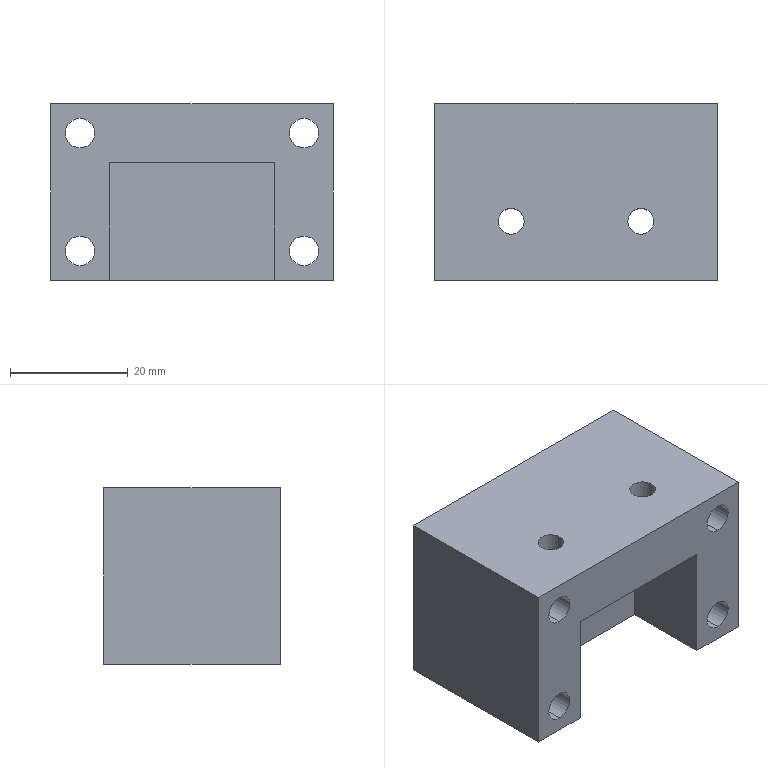Part | SolidWorks | features ICE 3, Extrusion 1 | 1 solid | 22 faces | box 48 x 30 x 30 mm | volume 32140 mm3 | cylinder 12 | plane 10 | commonest cylinder face diameters 5 x8 4.4 x4
STEP:
#1=CARTESIAN_POINT('',(0.01845,0.01653,0.0025));
#2=VERTEX_POINT('',#1);
#3=CARTESIAN_POINT('',(0.01845,0.01653,0.0075));
#4=VERTEX_POINT('',#3);
#5=CARTESIAN_POINT('',(0.01845,0.01653,0.005));
#6=DIRECTION('',(0.,1.,0.));
#7=DIRECTION('',(0.,0.,-1.));
#8=AXIS2_PLACEMENT_3D('',#5,#6,#7);
#9=CIRCLE('',#8,0.0025);
#10=EDGE_CURVE('',#2,#4,#9,.T.);
#11=ORIENTED_EDGE('',*,*,#10,.T.);
#12=CARTESIAN_POINT('',(0.01845,-0.01347,0.0075));
#13=VERTEX_POINT('',#12);
#14=CARTESIAN_POINT('',(0.01845,0.0236,0.0075));
#15=DIRECTION('',(0.,-1.,0.));
#16=VECTOR('',#15,1.);
#17=LINE('',#14,#16);
#18=EDGE_CURVE('',#4,#13,#17,.T.);
#19=ORIENTED_EDGE('',*,*,#18,.T.);
#20=CARTESIAN_POINT('',(0.01845,-0.01347,0.0025));
#21=VERTEX_POINT('',#20);
#22=CARTESIAN_POINT('',(0.01845,-0.01347,0.005));
#23=DIRECTION('',(0.,-1.,0.));
#24=DIRECTION('',(0.,0.,-1.));
#25=AXIS2_PLACEMENT_3D('',#22,#23,#24);
#26=CIRCLE('',#25,0.0025);
#27=EDGE_CURVE('',#13,#21,#26,.T.);
#28=ORIENTED_EDGE('',*,*,#27,.T.);
#29=CARTESIAN_POINT('',(0.01845,0.0236,0.0025));
#30=DIRECTION('',(0.,-1.,0.));
#31=VECTOR('',#30,1.);
#32=LINE('',#29,#31);
#33=EDGE_CURVE('',#2,#21,#32,.T.);
#34=ORIENTED_EDGE('',*,*,#33,.F.);
#35=EDGE_LOOP('',(#11,#19,#28,#34));
#36=FACE_OUTER_BOUND('',#35,.T.);
#37=CARTESIAN_POINT('',(0.01845,0.0236,0.005));
#38=DIRECTION('',(0.,-1.,0.));
#39=DIRECTION('',(0.,0.,-1.));
#40=AXIS2_PLACEMENT_3D('',#37,#38,#39);
#41=CYLINDRICAL_SURFACE('',#40,0.0025);
#42=ADVANCED_FACE('',(#36),#41,.F.);
#43=CARTESIAN_POINT('',(0.01845,0.01653,0.0225));
#44=VERTEX_POINT('',#43);
#45=CARTESIAN_POINT('',(0.01845,0.01653,0.0275));
#46=VERTEX_POINT('',#45);
#47=CARTESIAN_POINT('',(0.01845,0.01653,0.025));
#48=DIRECTION('',(0.,1.,0.));
#49=DIRECTION('',(0.,0.,-1.));
#50=AXIS2_PLACEMENT_3D('',#47,#48,#49);
#51=CIRCLE('',#50,0.0025);
#52=EDGE_CURVE('',#44,#46,#51,.T.);
#53=ORIENTED_EDGE('',*,*,#52,.T.);
#54=CARTESIAN_POINT('',(0.01845,-0.01347,0.0275));
#55=VERTEX_POINT('',#54);
#56=CARTESIAN_POINT('',(0.01845,0.0236,0.0275));
#57=DIRECTION('',(0.,-1.,0.));
#58=VECTOR('',#57,1.);
#59=LINE('',#56,#58);
#60=EDGE_CURVE('',#46,#55,#59,.T.);
#61=ORIENTED_EDGE('',*,*,#60,.T.);
#62=CARTESIAN_POINT('',(0.01845,-0.01347,0.0225));
#63=VERTEX_POINT('',#62);
#64=CARTESIAN_POINT('',(0.01845,-0.01347,0.025));
#65=DIRECTION('',(0.,-1.,0.));
#66=DIRECTION('',(0.,0.,-1.));
#67=AXIS2_PLACEMENT_3D('',#64,#65,#66);
#68=CIRCLE('',#67,0.0025);
#69=EDGE_CURVE('',#55,#63,#68,.T.);
#70=ORIENTED_EDGE('',*,*,#69,.T.);
#71=CARTESIAN_POINT('',(0.01845,0.0236,0.0225));
#72=DIRECTION('',(0.,-1.,0.));
#73=VECTOR('',#72,1.);
#74=LINE('',#71,#73);
#75=EDGE_CURVE('',#44,#63,#74,.T.);
#76=ORIENTED_EDGE('',*,*,#75,.F.);
#77=EDGE_LOOP('',(#53,#61,#70,#76));
#78=FACE_OUTER_BOUND('',#77,.T.);
#79=CARTESIAN_POINT('',(0.01845,0.0236,0.025));
#80=DIRECTION('',(0.,-1.,0.));
#81=DIRECTION('',(0.,0.,-1.));
#82=AXIS2_PLACEMENT_3D('',#79,#80,#81);
#83=CYLINDRICAL_SURFACE('',#82,0.0025);
#84=ADVANCED_FACE('',(#78),#83,.F.);
#85=CARTESIAN_POINT('',(-0.01955,0.01653,0.0225));
#86=VERTEX_POINT('',#85);
#87=CARTESIAN_POINT('',(-0.01955,0.01653,0.0275));
#88=VERTEX_POINT('',#87);
#89=CARTESIAN_POINT('',(-0.01955,0.01653,0.025));
#90=DIRECTION('',(0.,1.,0.));
#91=DIRECTION('',(0.,0.,-1.));
#92=AXIS2_PLACEMENT_3D('',#89,#90,#91);
#93=CIRCLE('',#92,0.0025);
#94=EDGE_CURVE('',#86,#88,#93,.T.);
#95=ORIENTED_EDGE('',*,*,#94,.T.);
#96=CARTESIAN_POINT('',(-0.01955,-0.01347,0.0275));
#97=VERTEX_POINT('',#96);
#98=CARTESIAN_POINT('',(-0.01955,0.0236,0.0275));
#99=DIRECTION('',(0.,-1.,0.));
#100=VECTOR('',#99,1.);
#101=LINE('',#98,#100);
#102=EDGE_CURVE('',#88,#97,#101,.T.);
#103=ORIENTED_EDGE('',*,*,#102,.T.);
#104=CARTESIAN_POINT('',(-0.01955,-0.01347,0.0225));
#105=VERTEX_POINT('',#104);
#106=CARTESIAN_POINT('',(-0.01955,-0.01347,0.025));
#107=DIRECTION('',(0.,-1.,0.));
#108=DIRECTION('',(0.,0.,-1.));
#109=AXIS2_PLACEMENT_3D('',#106,#107,#108);
#110=CIRCLE('',#109,0.0025);
#111=EDGE_CURVE('',#97,#105,#110,.T.);
#112=ORIENTED_EDGE('',*,*,#111,.T.);
#113=CARTESIAN_POINT('',(-0.01955,0.0236,0.0225));
#114=DIRECTION('',(0.,-1.,0.));
#115=VECTOR('',#114,1.);
#116=LINE('',#113,#115);
#117=EDGE_CURVE('',#86,#105,#116,.T.);
#118=ORIENTED_EDGE('',*,*,#117,.F.);
#119=EDGE_LOOP('',(#95,#103,#112,#118));
#120=FACE_OUTER_BOUND('',#119,.T.);
#121=CARTESIAN_POINT('',(-0.01955,0.0236,0.025));
#122=DIRECTION('',(0.,-1.,0.));
#123=DIRECTION('',(0.,0.,-1.));
#124=AXIS2_PLACEMENT_3D('',#121,#122,#123);
#125=CYLINDRICAL_SURFACE('',#124,0.0025);
#126=ADVANCED_FACE('',(#120),#125,.F.);
#127=CARTESIAN_POINT('',(-0.01955,0.01653,0.0025));
#128=VERTEX_POINT('',#127);
#129=CARTESIAN_POINT('',(-0.01955,0.01653,0.0075));
#130=VERTEX_POINT('',#129);
#131=CARTESIAN_POINT('',(-0.01955,0.01653,0.005));
#132=DIRECTION('',(0.,1.,0.));
#133=DIRECTION('',(0.,0.,-1.));
#134=AXIS2_PLACEMENT_3D('',#131,#132,#133);
#135=CIRCLE('',#134,0.0025);
#136=EDGE_CURVE('',#128,#130,#135,.T.);
#137=ORIENTED_EDGE('',*,*,#136,.T.);
#138=CARTESIAN_POINT('',(-0.01955,-0.01347,0.0075));
#139=VERTEX_POINT('',#138);
#140=CARTESIAN_POINT('',(-0.01955,0.0236,0.0075));
#141=DIRECTION('',(0.,-1.,0.));
#142=VECTOR('',#141,1.);
#143=LINE('',#140,#142);
#144=EDGE_CURVE('',#130,#139,#143,.T.);
#145=ORIENTED_EDGE('',*,*,#144,.T.);
#146=CARTESIAN_POINT('',(-0.01955,-0.01347,0.0025));
#147=VERTEX_POINT('',#146);
#148=CARTESIAN_POINT('',(-0.01955,-0.01347,0.005));
#149=DIRECTION('',(0.,-1.,0.));
#150=DIRECTION('',(0.,0.,-1.));
#151=AXIS2_PLACEMENT_3D('',#148,#149,#150);
#152=CIRCLE('',#151,0.0025);
#153=EDGE_CURVE('',#139,#147,#152,.T.);
#154=ORIENTED_EDGE('',*,*,#153,.T.);
#155=CARTESIAN_POINT('',(-0.01955,0.0236,0.0025));
#156=DIRECTION('',(0.,-1.,0.));
#157=VECTOR('',#156,1.);
#158=LINE('',#155,#157);
#159=EDGE_CURVE('',#128,#147,#158,.T.);
#160=ORIENTED_EDGE('',*,*,#159,.F.);
#161=EDGE_LOOP('',(#137,#145,#154,#160));
#162=FACE_OUTER_BOUND('',#161,.T.);
#163=CARTESIAN_POINT('',(-0.01955,0.0236,0.005));
#164=DIRECTION('',(0.,-1.,0.));
#165=DIRECTION('',(0.,0.,-1.));
#166=AXIS2_PLACEMENT_3D('',#163,#164,#165);
#167=CYLINDRICAL_SURFACE('',#166,0.0025);
#168=ADVANCED_FACE('',(#162),#167,.F.);
#169=CARTESIAN_POINT('',(0.008255,-0.003473,0.03));
#170=VERTEX_POINT('',#169);
#171=CARTESIAN_POINT('',(0.01265,-0.003473,0.03));
#172=VERTEX_POINT('',#171);
#173=CARTESIAN_POINT('',(0.01045,-0.003473,0.03));
#174=DIRECTION('',(0.,0.,1.));
#175=DIRECTION('',(1.,0.,0.));
#176=AXIS2_PLACEMENT_3D('',#173,#174,#175);
#177=CIRCLE('',#176,0.0022);
#178=EDGE_CURVE('',#170,#172,#177,.T.);
#179=ORIENTED_EDGE('',*,*,#178,.T.);
#180=CARTESIAN_POINT('',(0.01265,-0.003473,0.02));
#181=VERTEX_POINT('',#180);
#182=CARTESIAN_POINT('',(0.01265,-0.003473,0.04));
#183=DIRECTION('',(0.,0.,-1.));
#184=VECTOR('',#183,1.);
#185=LINE('',#182,#184);
#186=EDGE_CURVE('',#172,#181,#185,.T.);
#187=ORIENTED_EDGE('',*,*,#186,.T.);
#188=CARTESIAN_POINT('',(0.008255,-0.003473,0.02));
#189=VERTEX_POINT('',#188);
#190=CARTESIAN_POINT('',(0.01045,-0.003473,0.02));
#191=DIRECTION('',(0.,0.,-1.));
#192=DIRECTION('',(-1.,0.,0.));
#193=AXIS2_PLACEMENT_3D('',#190,#191,#192);
#194=CIRCLE('',#193,0.0022);
#195=EDGE_CURVE('',#181,#189,#194,.T.);
#196=ORIENTED_EDGE('',*,*,#195,.T.);
#197=CARTESIAN_POINT('',(0.008255,-0.003473,0.04));
#198=DIRECTION('',(0.,0.,-1.));
#199=VECTOR('',#198,1.);
#200=LINE('',#197,#199);
#201=EDGE_CURVE('',#170,#189,#200,.T.);
#202=ORIENTED_EDGE('',*,*,#201,.F.);
#203=EDGE_LOOP('',(#179,#187,#196,#202));
#204=FACE_OUTER_BOUND('',#203,.T.);
#205=CARTESIAN_POINT('',(0.01045,-0.003473,0.04));
#206=DIRECTION('',(0.,0.,-1.));
#207=DIRECTION('',(-1.,0.,0.));
#208=AXIS2_PLACEMENT_3D('',#205,#206,#207);
#209=CYLINDRICAL_SURFACE('',#208,0.0022);
#210=ADVANCED_FACE('',(#204),#209,.F.);
#211=CARTESIAN_POINT('',(-0.01375,-0.003473,0.03));
#212=VERTEX_POINT('',#211);
#213=CARTESIAN_POINT('',(-0.009345,-0.003473,0.03));
#214=VERTEX_POINT('',#213);
#215=CARTESIAN_POINT('',(-0.01155,-0.003473,0.03));
#216=DIRECTION('',(0.,0.,1.));
#217=DIRECTION('',(1.,0.,0.));
#218=AXIS2_PLACEMENT_3D('',#215,#216,#217);
#219=CIRCLE('',#218,0.0022);
#220=EDGE_CURVE('',#212,#214,#219,.T.);
#221=ORIENTED_EDGE('',*,*,#220,.T.);
#222=CARTESIAN_POINT('',(-0.009345,-0.003473,0.02));
#223=VERTEX_POINT('',#222);
#224=CARTESIAN_POINT('',(-0.009345,-0.003473,0.04));
#225=DIRECTION('',(0.,0.,-1.));
#226=VECTOR('',#225,1.);
#227=LINE('',#224,#226);
#228=EDGE_CURVE('',#214,#223,#227,.T.);
#229=ORIENTED_EDGE('',*,*,#228,.T.);
#230=CARTESIAN_POINT('',(-0.01375,-0.003473,0.02));
#231=VERTEX_POINT('',#230);
#232=CARTESIAN_POINT('',(-0.01155,-0.003473,0.02));
#233=DIRECTION('',(0.,0.,-1.));
#234=DIRECTION('',(-1.,0.,0.));
#235=AXIS2_PLACEMENT_3D('',#232,#233,#234);
#236=CIRCLE('',#235,0.0022);
#237=EDGE_CURVE('',#223,#231,#236,.T.);
#238=ORIENTED_EDGE('',*,*,#237,.T.);
#239=CARTESIAN_POINT('',(-0.01375,-0.003473,0.04));
#240=DIRECTION('',(0.,0.,-1.));
#241=VECTOR('',#240,1.);
#242=LINE('',#239,#241);
#243=EDGE_CURVE('',#212,#231,#242,.T.);
#244=ORIENTED_EDGE('',*,*,#243,.F.);
#245=EDGE_LOOP('',(#221,#229,#238,#244));
#246=FACE_OUTER_BOUND('',#245,.T.);
#247=CARTESIAN_POINT('',(-0.01155,-0.003473,0.04));
#248=DIRECTION('',(0.,0.,-1.));
#249=DIRECTION('',(-1.,0.,0.));
#250=AXIS2_PLACEMENT_3D('',#247,#248,#249);
#251=CYLINDRICAL_SURFACE('',#250,0.0022);
#252=ADVANCED_FACE('',(#246),#251,.F.);
#253=CARTESIAN_POINT('',(-0.02455,0.01653,0.));
#254=VERTEX_POINT('',#253);
#255=CARTESIAN_POINT('',(-0.02455,-0.01347,0.));
#256=VERTEX_POINT('',#255);
#257=CARTESIAN_POINT('',(-0.02455,0.01653,0.));
#258=DIRECTION('',(0.,-1.,0.));
#259=VECTOR('',#258,1.);
#260=LINE('',#257,#259);
#261=EDGE_CURVE('',#254,#256,#260,.T.);
#262=ORIENTED_EDGE('',*,*,#261,.T.);
#263=CARTESIAN_POINT('',(-0.02455,-0.01347,0.03));
#264=VERTEX_POINT('',#263);
#265=CARTESIAN_POINT('',(-0.02455,-0.01347,0.03));
#266=DIRECTION('',(0.,0.,-1.));
#267=VECTOR('',#266,1.);
#268=LINE('',#265,#267);
#269=EDGE_CURVE('',#264,#256,#268,.T.);
#270=ORIENTED_EDGE('',*,*,#269,.F.);
#271=CARTESIAN_POINT('',(-0.02455,0.01653,0.03));
#272=VERTEX_POINT('',#271);
#273=CARTESIAN_POINT('',(-0.02455,0.01653,0.03));
#274=DIRECTION('',(0.,-1.,0.));
#275=VECTOR('',#274,1.);
#276=LINE('',#273,#275);
#277=EDGE_CURVE('',#272,#264,#276,.T.);
#278=ORIENTED_EDGE('',*,*,#277,.F.);
#279=CARTESIAN_POINT('',(-0.02455,0.01653,0.03));
#280=DIRECTION('',(0.,0.,-1.));
#281=VECTOR('',#280,1.);
#282=LINE('',#279,#281);
#283=EDGE_CURVE('',#272,#254,#282,.T.);
#284=ORIENTED_EDGE('',*,*,#283,.T.);
#285=EDGE_LOOP('',(#262,#270,#278,#284));
#286=FACE_OUTER_BOUND('',#285,.T.);
#287=CARTESIAN_POINT('',(-0.02455,0.01653,0.03));
#288=DIRECTION('',(1.,0.,0.));
#289=DIRECTION('',(0.,1.,0.));
#290=AXIS2_PLACEMENT_3D('',#287,#288,#289);
#291=PLANE('',#290);
#292=ADVANCED_FACE('',(#286),#291,.F.);
#293=CARTESIAN_POINT('',(0.01845,-0.01347,0.005));
#294=DIRECTION('',(0.,-1.,0.));
#295=DIRECTION('',(0.,0.,-1.));
#296=AXIS2_PLACEMENT_3D('',#293,#294,#295);
#297=CIRCLE('',#296,0.0025);
#298=EDGE_CURVE('',#21,#13,#297,.T.);
#299=ORIENTED_EDGE('',*,*,#298,.F.);
#300=ORIENTED_EDGE('',*,*,#27,.F.);
#301=EDGE_LOOP('',(#299,#300));
#302=FACE_BOUND('',#301,.T.);
#303=CARTESIAN_POINT('',(0.01845,-0.01347,0.025));
#304=DIRECTION('',(0.,-1.,0.));
#305=DIRECTION('',(0.,0.,-1.));
#306=AXIS2_PLACEMENT_3D('',#303,#304,#305);
#307=CIRCLE('',#306,0.0025);
#308=EDGE_CURVE('',#63,#55,#307,.T.);
#309=ORIENTED_EDGE('',*,*,#308,.F.);
#310=ORIENTED_EDGE('',*,*,#69,.F.);
#311=EDGE_LOOP('',(#309,#310));
#312=FACE_BOUND('',#311,.T.);
#313=CARTESIAN_POINT('',(-0.01955,-0.01347,0.025));
#314=DIRECTION('',(0.,-1.,0.));
#315=DIRECTION('',(0.,0.,-1.));
#316=AXIS2_PLACEMENT_3D('',#313,#314,#315);
#317=CIRCLE('',#316,0.0025);
#318=EDGE_CURVE('',#105,#97,#317,.T.);
#319=ORIENTED_EDGE('',*,*,#318,.F.);
#320=ORIENTED_EDGE('',*,*,#111,.F.);
#321=EDGE_LOOP('',(#319,#320));
#322=FACE_BOUND('',#321,.T.);
#323=CARTESIAN_POINT('',(-0.01955,-0.01347,0.005));
#324=DIRECTION('',(0.,-1.,0.));
#325=DIRECTION('',(0.,0.,-1.));
#326=AXIS2_PLACEMENT_3D('',#323,#324,#325);
#327=CIRCLE('',#326,0.0025);
#328=EDGE_CURVE('',#147,#139,#327,.T.);
#329=ORIENTED_EDGE('',*,*,#328,.F.);
#330=ORIENTED_EDGE('',*,*,#153,.F.);
#331=EDGE_LOOP('',(#329,#330));
#332=FACE_BOUND('',#331,.T.);
#333=CARTESIAN_POINT('',(0.01345,-0.01347,0.02));
#334=VERTEX_POINT('',#333);
#335=CARTESIAN_POINT('',(-0.01455,-0.01347,0.02));
#336=VERTEX_POINT('',#335);
#337=CARTESIAN_POINT('',(0.01345,-0.01347,0.02));
#338=DIRECTION('',(-1.,0.,0.));
#339=VECTOR('',#338,1.);
#340=LINE('',#337,#339);
#341=EDGE_CURVE('',#334,#336,#340,.T.);
#342=ORIENTED_EDGE('',*,*,#341,.F.);
#343=CARTESIAN_POINT('',(0.01345,-0.01347,0.));
#344=VERTEX_POINT('',#343);
#345=CARTESIAN_POINT('',(0.01345,-0.01347,0.02));
#346=DIRECTION('',(0.,0.,-1.));
#347=VECTOR('',#346,1.);
#348=LINE('',#345,#347);
#349=EDGE_CURVE('',#334,#344,#348,.T.);
#350=ORIENTED_EDGE('',*,*,#349,.T.);
#351=CARTESIAN_POINT('',(0.02345,-0.01347,0.));
#352=VERTEX_POINT('',#351);
#353=CARTESIAN_POINT('',(-0.02455,-0.01347,0.));
#354=DIRECTION('',(1.,0.,0.));
#355=VECTOR('',#354,1.);
#356=LINE('',#353,#355);
#357=EDGE_CURVE('',#344,#352,#356,.T.);
#358=ORIENTED_EDGE('',*,*,#357,.T.);
#359=CARTESIAN_POINT('',(0.02345,-0.01347,0.03));
#360=VERTEX_POINT('',#359);
#361=CARTESIAN_POINT('',(0.02345,-0.01347,0.03));
#362=DIRECTION('',(0.,0.,-1.));
#363=VECTOR('',#362,1.);
#364=LINE('',#361,#363);
#365=EDGE_CURVE('',#360,#352,#364,.T.);
#366=ORIENTED_EDGE('',*,*,#365,.F.);
#367=CARTESIAN_POINT('',(-0.02455,-0.01347,0.03));
#368=DIRECTION('',(1.,0.,0.));
#369=VECTOR('',#368,1.);
#370=LINE('',#367,#369);
#371=EDGE_CURVE('',#264,#360,#370,.T.);
#372=ORIENTED_EDGE('',*,*,#371,.F.);
#373=ORIENTED_EDGE('',*,*,#269,.T.);
#374=CARTESIAN_POINT('',(-0.01455,-0.01347,0.));
#375=VERTEX_POINT('',#374);
#376=CARTESIAN_POINT('',(-0.02455,-0.01347,0.));
#377=DIRECTION('',(1.,0.,0.));
#378=VECTOR('',#377,1.);
#379=LINE('',#376,#378);
#380=EDGE_CURVE('',#256,#375,#379,.T.);
#381=ORIENTED_EDGE('',*,*,#380,.T.);
#382=CARTESIAN_POINT('',(-0.01455,-0.01347,0.02));
#383=DIRECTION('',(0.,0.,-1.));
#384=VECTOR('',#383,1.);
#385=LINE('',#382,#384);
#386=EDGE_CURVE('',#336,#375,#385,.T.);
#387=ORIENTED_EDGE('',*,*,#386,.F.);
#388=EDGE_LOOP('',(#342,#350,#358,#366,#372,#373,#381,#387));
#389=FACE_OUTER_BOUND('',#388,.T.);
#390=CARTESIAN_POINT('',(-0.02455,-0.01347,0.03));
#391=DIRECTION('',(0.,1.,0.));
#392=DIRECTION('',(0.,0.,1.));
#393=AXIS2_PLACEMENT_3D('',#390,#391,#392);
#394=PLANE('',#393);
#395=ADVANCED_FACE('',(#302,#312,#322,#332,#389),#394,.F.);
#396=CARTESIAN_POINT('',(0.02345,0.01653,0.));
#397=VERTEX_POINT('',#396);
#398=CARTESIAN_POINT('',(0.02345,0.01653,0.));
#399=DIRECTION('',(0.,1.,0.));
#400=VECTOR('',#399,1.);
#401=LINE('',#398,#400);
#402=EDGE_CURVE('',#352,#397,#401,.T.);
#403=ORIENTED_EDGE('',*,*,#402,.T.);
#404=CARTESIAN_POINT('',(0.02345,0.01653,0.03));
#405=VERTEX_POINT('',#404);
#406=CARTESIAN_POINT('',(0.02345,0.01653,0.03));
#407=DIRECTION('',(0.,0.,-1.));
#408=VECTOR('',#407,1.);
#409=LINE('',#406,#408);
#410=EDGE_CURVE('',#405,#397,#409,.T.);
#411=ORIENTED_EDGE('',*,*,#410,.F.);
#412=CARTESIAN_POINT('',(0.02345,0.01653,0.03));
#413=DIRECTION('',(0.,1.,0.));
#414=VECTOR('',#413,1.);
#415=LINE('',#412,#414);
#416=EDGE_CURVE('',#360,#405,#415,.T.);
#417=ORIENTED_EDGE('',*,*,#416,.F.);
#418=ORIENTED_EDGE('',*,*,#365,.T.);
#419=EDGE_LOOP('',(#403,#411,#417,#418));
#420=FACE_OUTER_BOUND('',#419,.T.);
#421=CARTESIAN_POINT('',(0.02345,0.01653,0.03));
#422=DIRECTION('',(-1.,0.,0.));
#423=DIRECTION('',(0.,-1.,0.));
#424=AXIS2_PLACEMENT_3D('',#421,#422,#423);
#425=PLANE('',#424);
#426=ADVANCED_FACE('',(#420),#425,.F.);
#427=ORIENTED_EDGE('',*,*,#10,.F.);
#428=CARTESIAN_POINT('',(0.01845,0.01653,0.005));
#429=DIRECTION('',(0.,1.,0.));
#430=DIRECTION('',(0.,0.,-1.));
#431=AXIS2_PLACEMENT_3D('',#428,#429,#430);
#432=CIRCLE('',#431,0.0025);
#433=EDGE_CURVE('',#4,#2,#432,.T.);
#434=ORIENTED_EDGE('',*,*,#433,.F.);
#435=EDGE_LOOP('',(#427,#434));
#436=FACE_BOUND('',#435,.T.);
#437=ORIENTED_EDGE('',*,*,#52,.F.);
#438=CARTESIAN_POINT('',(0.01845,0.01653,0.025));
#439=DIRECTION('',(0.,1.,0.));
#440=DIRECTION('',(0.,0.,-1.));
#441=AXIS2_PLACEMENT_3D('',#438,#439,#440);
#442=CIRCLE('',#441,0.0025);
#443=EDGE_CURVE('',#46,#44,#442,.T.);
#444=ORIENTED_EDGE('',*,*,#443,.F.);
#445=EDGE_LOOP('',(#437,#444));
#446=FACE_BOUND('',#445,.T.);
#447=ORIENTED_EDGE('',*,*,#94,.F.);
#448=CARTESIAN_POINT('',(-0.01955,0.01653,0.025));
#449=DIRECTION('',(0.,1.,0.));
#450=DIRECTION('',(0.,0.,-1.));
#451=AXIS2_PLACEMENT_3D('',#448,#449,#450);
#452=CIRCLE('',#451,0.0025);
#453=EDGE_CURVE('',#88,#86,#452,.T.);
#454=ORIENTED_EDGE('',*,*,#453,.F.);
#455=EDGE_LOOP('',(#447,#454));
#456=FACE_BOUND('',#455,.T.);
#457=ORIENTED_EDGE('',*,*,#136,.F.);
#458=CARTESIAN_POINT('',(-0.01955,0.01653,0.005));
#459=DIRECTION('',(0.,1.,0.));
#460=DIRECTION('',(0.,0.,-1.));
#461=AXIS2_PLACEMENT_3D('',#458,#459,#460);
#462=CIRCLE('',#461,0.0025);
#463=EDGE_CURVE('',#130,#128,#462,.T.);
#464=ORIENTED_EDGE('',*,*,#463,.F.);
#465=EDGE_LOOP('',(#457,#464));
#466=FACE_BOUND('',#465,.T.);
#467=CARTESIAN_POINT('',(-0.02455,0.01653,0.));
#468=DIRECTION('',(-1.,0.,0.));
#469=VECTOR('',#468,1.);
#470=LINE('',#467,#469);
#471=EDGE_CURVE('',#397,#254,#470,.T.);
#472=ORIENTED_EDGE('',*,*,#471,.T.);
#473=ORIENTED_EDGE('',*,*,#283,.F.);
#474=CARTESIAN_POINT('',(-0.02455,0.01653,0.03));
#475=DIRECTION('',(-1.,0.,0.));
#476=VECTOR('',#475,1.);
#477=LINE('',#474,#476);
#478=EDGE_CURVE('',#405,#272,#477,.T.);
#479=ORIENTED_EDGE('',*,*,#478,.F.);
#480=ORIENTED_EDGE('',*,*,#410,.T.);
#481=EDGE_LOOP('',(#472,#473,#479,#480));
#482=FACE_OUTER_BOUND('',#481,.T.);
#483=CARTESIAN_POINT('',(-0.02455,0.01653,0.03));
#484=DIRECTION('',(0.,-1.,0.));
#485=DIRECTION('',(0.,0.,-1.));
#486=AXIS2_PLACEMENT_3D('',#483,#484,#485);
#487=PLANE('',#486);
#488=ADVANCED_FACE('',(#436,#446,#456,#466,#482),#487,.F.);
#489=ORIENTED_EDGE('',*,*,#178,.F.);
#490=CARTESIAN_POINT('',(0.01045,-0.003473,0.03));
#491=DIRECTION('',(0.,0.,1.));
#492=DIRECTION('',(1.,0.,0.));
#493=AXIS2_PLACEMENT_3D('',#490,#491,#492);
#494=CIRCLE('',#493,0.0022);
#495=EDGE_CURVE('',#172,#170,#494,.T.);
#496=ORIENTED_EDGE('',*,*,#495,.F.);
#497=EDGE_LOOP('',(#489,#496));
#498=FACE_BOUND('',#497,.T.);
#499=ORIENTED_EDGE('',*,*,#220,.F.);
#500=CARTESIAN_POINT('',(-0.01155,-0.003473,0.03));
#501=DIRECTION('',(0.,0.,1.));
#502=DIRECTION('',(1.,0.,0.));
#503=AXIS2_PLACEMENT_3D('',#500,#501,#502);
#504=CIRCLE('',#503,0.0022);
#505=EDGE_CURVE('',#214,#212,#504,.T.);
#506=ORIENTED_EDGE('',*,*,#505,.F.);
#507=EDGE_LOOP('',(#499,#506));
#508=FACE_BOUND('',#507,.T.);
#509=ORIENTED_EDGE('',*,*,#277,.T.);
#510=ORIENTED_EDGE('',*,*,#371,.T.);
#511=ORIENTED_EDGE('',*,*,#416,.T.);
#512=ORIENTED_EDGE('',*,*,#478,.T.);
#513=EDGE_LOOP('',(#509,#510,#511,#512));
#514=FACE_OUTER_BOUND('',#513,.T.);
#515=CARTESIAN_POINT('',(0.,0.,0.03));
#516=DIRECTION('',(0.,0.,1.));
#517=DIRECTION('',(1.,0.,0.));
#518=AXIS2_PLACEMENT_3D('',#515,#516,#517);
#519=PLANE('',#518);
#520=ADVANCED_FACE('',(#498,#508,#514),#519,.T.);
#521=ORIENTED_EDGE('',*,*,#357,.F.);
#522=CARTESIAN_POINT('',(0.01345,0.001527,0.));
#523=VERTEX_POINT('',#522);
#524=CARTESIAN_POINT('',(0.01345,-0.01347,0.));
#525=DIRECTION('',(0.,-1.,0.));
#526=VECTOR('',#525,1.);
#527=LINE('',#524,#526);
#528=EDGE_CURVE('',#523,#344,#527,.T.);
#529=ORIENTED_EDGE('',*,*,#528,.F.);
#530=CARTESIAN_POINT('',(-0.01455,0.001527,0.));
#531=VERTEX_POINT('',#530);
#532=CARTESIAN_POINT('',(0.01345,0.001527,0.));
#533=DIRECTION('',(1.,0.,0.));
#534=VECTOR('',#533,1.);
#535=LINE('',#532,#534);
#536=EDGE_CURVE('',#531,#523,#535,.T.);
#537=ORIENTED_EDGE('',*,*,#536,.F.);
#538=CARTESIAN_POINT('',(-0.01455,-0.01347,0.));
#539=DIRECTION('',(0.,1.,0.));
#540=VECTOR('',#539,1.);
#541=LINE('',#538,#540);
#542=EDGE_CURVE('',#375,#531,#541,.T.);
#543=ORIENTED_EDGE('',*,*,#542,.F.);
#544=ORIENTED_EDGE('',*,*,#380,.F.);
#545=ORIENTED_EDGE('',*,*,#261,.F.);
#546=ORIENTED_EDGE('',*,*,#471,.F.);
#547=ORIENTED_EDGE('',*,*,#402,.F.);
#548=EDGE_LOOP('',(#521,#529,#537,#543,#544,#545,#546,#547));
#549=FACE_OUTER_BOUND('',#548,.T.);
#550=CARTESIAN_POINT('',(0.,0.,0.));
#551=DIRECTION('',(0.,0.,1.));
#552=DIRECTION('',(1.,0.,0.));
#553=AXIS2_PLACEMENT_3D('',#550,#551,#552);
#554=PLANE('',#553);
#555=ADVANCED_FACE('',(#549),#554,.F.);
#556=ORIENTED_EDGE('',*,*,#528,.T.);
#557=ORIENTED_EDGE('',*,*,#349,.F.);
#558=CARTESIAN_POINT('',(0.01345,0.001527,0.02));
#559=VERTEX_POINT('',#558);
#560=CARTESIAN_POINT('',(0.01345,-0.01347,0.02));
#561=DIRECTION('',(0.,-1.,0.));
#562=VECTOR('',#561,1.);
#563=LINE('',#560,#562);
#564=EDGE_CURVE('',#559,#334,#563,.T.);
#565=ORIENTED_EDGE('',*,*,#564,.F.);
#566=CARTESIAN_POINT('',(0.01345,0.001527,0.02));
#567=DIRECTION('',(0.,0.,-1.));
#568=VECTOR('',#567,1.);
#569=LINE('',#566,#568);
#570=EDGE_CURVE('',#559,#523,#569,.T.);
#571=ORIENTED_EDGE('',*,*,#570,.T.);
#572=EDGE_LOOP('',(#556,#557,#565,#571));
#573=FACE_OUTER_BOUND('',#572,.T.);
#574=CARTESIAN_POINT('',(0.01345,-0.01347,0.02));
#575=DIRECTION('',(1.,0.,0.));
#576=DIRECTION('',(0.,1.,0.));
#577=AXIS2_PLACEMENT_3D('',#574,#575,#576);
#578=PLANE('',#577);
#579=ADVANCED_FACE('',(#573),#578,.F.);
#580=ORIENTED_EDGE('',*,*,#536,.T.);
#581=ORIENTED_EDGE('',*,*,#570,.F.);
#582=CARTESIAN_POINT('',(-0.01455,0.001527,0.02));
#583=VERTEX_POINT('',#582);
#584=CARTESIAN_POINT('',(0.01345,0.001527,0.02));
#585=DIRECTION('',(1.,0.,0.));
#586=VECTOR('',#585,1.);
#587=LINE('',#584,#586);
#588=EDGE_CURVE('',#583,#559,#587,.T.);
#589=ORIENTED_EDGE('',*,*,#588,.F.);
#590=CARTESIAN_POINT('',(-0.01455,0.001527,0.02));
#591=DIRECTION('',(0.,0.,-1.));
#592=VECTOR('',#591,1.);
#593=LINE('',#590,#592);
#594=EDGE_CURVE('',#583,#531,#593,.T.);
#595=ORIENTED_EDGE('',*,*,#594,.T.);
#596=EDGE_LOOP('',(#580,#581,#589,#595));
#597=FACE_OUTER_BOUND('',#596,.T.);
#598=CARTESIAN_POINT('',(0.01345,0.001527,0.02));
#599=DIRECTION('',(0.,1.,0.));
#600=DIRECTION('',(0.,0.,1.));
#601=AXIS2_PLACEMENT_3D('',#598,#599,#600);
#602=PLANE('',#601);
#603=ADVANCED_FACE('',(#597),#602,.F.);
#604=ORIENTED_EDGE('',*,*,#542,.T.);
#605=ORIENTED_EDGE('',*,*,#594,.F.);
#606=CARTESIAN_POINT('',(-0.01455,-0.01347,0.02));
#607=DIRECTION('',(0.,1.,0.));
#608=VECTOR('',#607,1.);
#609=LINE('',#606,#608);
#610=EDGE_CURVE('',#336,#583,#609,.T.);
#611=ORIENTED_EDGE('',*,*,#610,.F.);
#612=ORIENTED_EDGE('',*,*,#386,.T.);
#613=EDGE_LOOP('',(#604,#605,#611,#612));
#614=FACE_OUTER_BOUND('',#613,.T.);
#615=CARTESIAN_POINT('',(-0.01455,-0.01347,0.02));
#616=DIRECTION('',(-1.,0.,0.));
#617=DIRECTION('',(0.,0.,1.));
#618=AXIS2_PLACEMENT_3D('',#615,#616,#617);
#619=PLANE('',#618);
#620=ADVANCED_FACE('',(#614),#619,.F.);
#621=CARTESIAN_POINT('',(0.01045,-0.003473,0.02));
#622=DIRECTION('',(0.,0.,-1.));
#623=DIRECTION('',(-1.,0.,0.));
#624=AXIS2_PLACEMENT_3D('',#621,#622,#623);
#625=CIRCLE('',#624,0.0022);
#626=EDGE_CURVE('',#189,#181,#625,.T.);
#627=ORIENTED_EDGE('',*,*,#626,.F.);
#628=ORIENTED_EDGE('',*,*,#195,.F.);
#629=EDGE_LOOP('',(#627,#628));
#630=FACE_BOUND('',#629,.T.);
#631=CARTESIAN_POINT('',(-0.01155,-0.003473,0.02));
#632=DIRECTION('',(0.,0.,-1.));
#633=DIRECTION('',(-1.,0.,0.));
#634=AXIS2_PLACEMENT_3D('',#631,#632,#633);
#635=CIRCLE('',#634,0.0022);
#636=EDGE_CURVE('',#231,#223,#635,.T.);
#637=ORIENTED_EDGE('',*,*,#636,.F.);
#638=ORIENTED_EDGE('',*,*,#237,.F.);
#639=EDGE_LOOP('',(#637,#638));
#640=FACE_BOUND('',#639,.T.);
#641=ORIENTED_EDGE('',*,*,#564,.T.);
#642=ORIENTED_EDGE('',*,*,#341,.T.);
#643=ORIENTED_EDGE('',*,*,#610,.T.);
#644=ORIENTED_EDGE('',*,*,#588,.T.);
#645=EDGE_LOOP('',(#641,#642,#643,#644));
#646=FACE_OUTER_BOUND('',#645,.T.);
#647=CARTESIAN_POINT('',(0.,0.,0.02));
#648=DIRECTION('',(0.,0.,1.));
#649=DIRECTION('',(1.,0.,0.));
#650=AXIS2_PLACEMENT_3D('',#647,#648,#649);
#651=PLANE('',#650);
#652=ADVANCED_FACE('',(#630,#640,#646),#651,.F.);
#653=ORIENTED_EDGE('',*,*,#228,.F.);
#654=ORIENTED_EDGE('',*,*,#505,.T.);
#655=ORIENTED_EDGE('',*,*,#243,.T.);
#656=ORIENTED_EDGE('',*,*,#636,.T.);
#657=EDGE_LOOP('',(#653,#654,#655,#656));
#658=FACE_OUTER_BOUND('',#657,.T.);
#659=CARTESIAN_POINT('',(-0.01155,-0.003473,0.04));
#660=DIRECTION('',(0.,0.,-1.));
#661=DIRECTION('',(-1.,0.,0.));
#662=AXIS2_PLACEMENT_3D('',#659,#660,#661);
#663=CYLINDRICAL_SURFACE('',#662,0.0022);
#664=ADVANCED_FACE('',(#658),#663,.F.);
#665=ORIENTED_EDGE('',*,*,#186,.F.);
#666=ORIENTED_EDGE('',*,*,#495,.T.);
#667=ORIENTED_EDGE('',*,*,#201,.T.);
#668=ORIENTED_EDGE('',*,*,#626,.T.);
#669=EDGE_LOOP('',(#665,#666,#667,#668));
#670=FACE_OUTER_BOUND('',#669,.T.);
#671=CARTESIAN_POINT('',(0.01045,-0.003473,0.04));
#672=DIRECTION('',(0.,0.,-1.));
#673=DIRECTION('',(-1.,0.,0.));
#674=AXIS2_PLACEMENT_3D('',#671,#672,#673);
#675=CYLINDRICAL_SURFACE('',#674,0.0022);
#676=ADVANCED_FACE('',(#670),#675,.F.);
#677=ORIENTED_EDGE('',*,*,#144,.F.);
#678=ORIENTED_EDGE('',*,*,#463,.T.);
#679=ORIENTED_EDGE('',*,*,#159,.T.);
#680=ORIENTED_EDGE('',*,*,#328,.T.);
#681=EDGE_LOOP('',(#677,#678,#679,#680));
#682=FACE_OUTER_BOUND('',#681,.T.);
#683=CARTESIAN_POINT('',(-0.01955,0.0236,0.005));
#684=DIRECTION('',(0.,-1.,0.));
#685=DIRECTION('',(0.,0.,-1.));
#686=AXIS2_PLACEMENT_3D('',#683,#684,#685);
#687=CYLINDRICAL_SURFACE('',#686,0.0025);
#688=ADVANCED_FACE('',(#682),#687,.F.);
#689=ORIENTED_EDGE('',*,*,#102,.F.);
#690=ORIENTED_EDGE('',*,*,#453,.T.);
#691=ORIENTED_EDGE('',*,*,#117,.T.);
#692=ORIENTED_EDGE('',*,*,#318,.T.);
#693=EDGE_LOOP('',(#689,#690,#691,#692));
#694=FACE_OUTER_BOUND('',#693,.T.);
#695=CARTESIAN_POINT('',(-0.01955,0.0236,0.025));
#696=DIRECTION('',(0.,-1.,0.));
#697=DIRECTION('',(0.,0.,-1.));
#698=AXIS2_PLACEMENT_3D('',#695,#696,#697);
#699=CYLINDRICAL_SURFACE('',#698,0.0025);
#700=ADVANCED_FACE('',(#694),#699,.F.);
#701=ORIENTED_EDGE('',*,*,#60,.F.);
#702=ORIENTED_EDGE('',*,*,#443,.T.);
#703=ORIENTED_EDGE('',*,*,#75,.T.);
#704=ORIENTED_EDGE('',*,*,#308,.T.);
#705=EDGE_LOOP('',(#701,#702,#703,#704));
#706=FACE_OUTER_BOUND('',#705,.T.);
#707=CARTESIAN_POINT('',(0.01845,0.0236,0.025));
#708=DIRECTION('',(0.,-1.,0.));
#709=DIRECTION('',(0.,0.,-1.));
#710=AXIS2_PLACEMENT_3D('',#707,#708,#709);
#711=CYLINDRICAL_SURFACE('',#710,0.0025);
#712=ADVANCED_FACE('',(#706),#711,.F.);
#713=ORIENTED_EDGE('',*,*,#18,.F.);
#714=ORIENTED_EDGE('',*,*,#433,.T.);
#715=ORIENTED_EDGE('',*,*,#33,.T.);
#716=ORIENTED_EDGE('',*,*,#298,.T.);
#717=EDGE_LOOP('',(#713,#714,#715,#716));
#718=FACE_OUTER_BOUND('',#717,.T.);
#719=CARTESIAN_POINT('',(0.01845,0.0236,0.005));
#720=DIRECTION('',(0.,-1.,0.));
#721=DIRECTION('',(0.,0.,-1.));
#722=AXIS2_PLACEMENT_3D('',#719,#720,#721);
#723=CYLINDRICAL_SURFACE('',#722,0.0025);
#724=ADVANCED_FACE('',(#718),#723,.F.);
#725=CLOSED_SHELL('',(#42,#84,#126,#168,#210,#252,#292,#395,#426,#488,#520,#555,#579,#603,#620,#652,#664,#676,#688,#700,#712,#724));
#726=MANIFOLD_SOLID_BREP('',#725);
#727=CARTESIAN_POINT('',(0.,0.,0.));
#728=DIRECTION('',(0.,0.,1.));
#729=DIRECTION('',(1.,0.,0.));
#730=AXIS2_PLACEMENT_3D('',#727,#728,#729);
#731=(LENGTH_UNIT()NAMED_UNIT(*)SI_UNIT($,.METRE.));
#732=UNCERTAINTY_MEASURE_WITH_UNIT(LENGTH_MEASURE(0.00001),#731,'','');
#733=(NAMED_UNIT(*)PLANE_ANGLE_UNIT()SI_UNIT($,.RADIAN.));
#734=(NAMED_UNIT(*)SI_UNIT($,.STERADIAN.)SOLID_ANGLE_UNIT());
#735=(GEOMETRIC_REPRESENTATION_CONTEXT(3)GLOBAL_UNCERTAINTY_ASSIGNED_CONTEXT((#732))GLOBAL_UNIT_ASSIGNED_CONTEXT((#731,#733,#734))REPRESENTATION_CONTEXT('',''));
#736=ADVANCED_BREP_SHAPE_REPRESENTATION('',(#726,#730),#735);